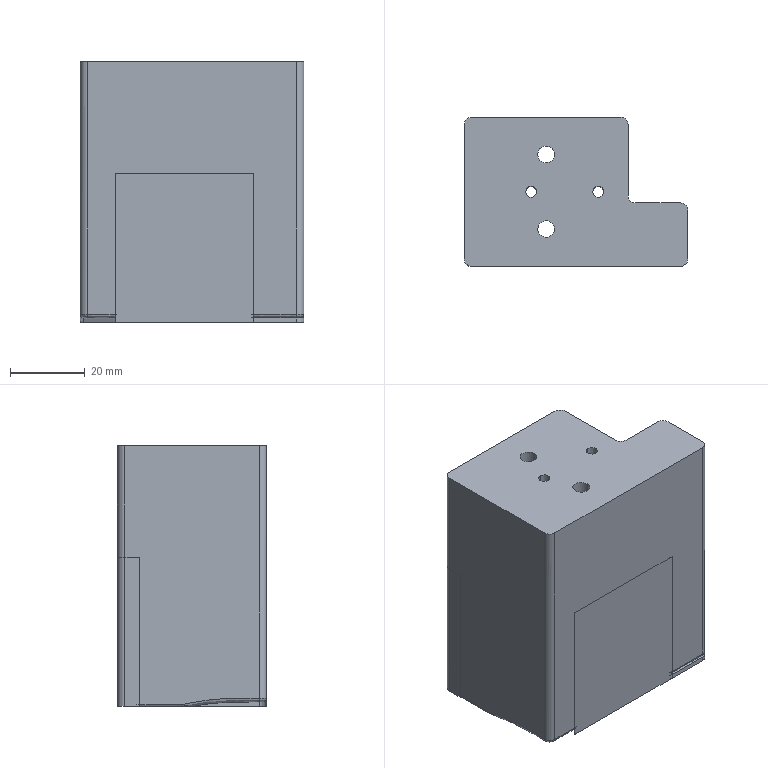NC program | NX | posted with a generic post | part box 60.004 x 40.015 x 70 mm
Lines 1319 to 2490 of 2490:
(ZLEVEL_PROFILE_COPY , TOOL : D6R0.5)
N2612 T08 M6
N2614 G54
N2616 G17 G0 G90 X-39.204 Y31.66 B0. C0. S9500 M3
N2618 G43 Z30. H8
N2620 Z1.491
N2622 G94 G1 Z-0.009 F1000.
N2624 X-38.808 Y30.909
N2626 G3 X-38.3 Y30.589 R0.6
N2628 X-35. Y30.711 R21.969 F3000.
N2630 G1 X35.
N2632 G3 X38.301 Y30.583 R28.78
N2634 G1 Y30.622 Z-0.014
N2636 Y30.645 Z-0.018
N2638 G2 X35. Y30.802 R29.046
N2640 G1 X-35.
N2642 G2 X-38.3 Y30.657 R19.705
N2644 G1 Y30.696 Z-0.024
N2646 Y30.722 Z-0.029
N2648 G3 X-35. Y30.878 R17.937
N2650 G1 X35.
N2652 G3 X38.3 Y30.71 R25.062
N2654 G1 Y30.75 Z-0.035
N2656 Y30.766 Z-0.042
N2658 G2 X35. Y30.954 R25.313
N2660 G1 X-35.
N2662 G2 X-38.3 Y30.78 R16.894
N2664 G1 Y30.838 Z-0.049
N2666 Y30.851 Z-0.057
N2668 G3 X-35. Y31.03 R17.218
N2670 G1 X35.
N2672 G3 X38.3 Y30.835 R25.117
N2674 G1 Y30.892 Z-0.066
N2676 Y30.914 Z-0.075
N2678 G2 X35. Y31.107 R26.565
N2680 G1 X-35.
N2682 G2 X-38.3 Y30.934 R19.629
N2684 G1 Y30.99 Z-0.085
N2686 Y31.028 Z-0.095
N2688 G3 X-35. Y31.184 R20.824
N2690 G1 X35.
N2692 X35.591 Y31.116
N2694 X38.3 Y31.005
N2696 Y31.052 Z-0.107
N2698 Y31.092 Z-0.119
N2700 G2 X35. Y31.262 R23.577
N2702 G1 X-35.
N2704 G2 X-38.3 Y31.107 R20.444
N2706 G1 Y31.15 Z-0.133
N2708 Y31.193 Z-0.146
N2710 G3 X-35. Y31.343 R22.3
N2712 G1 X35.
N2714 G3 X38.3 Y31.183 R24.663
N2716 G1 Y31.235 Z-0.162
N2718 Y31.286 Z-0.178
N2720 G2 X35. Y31.426 R29.09
N2722 G1 X-35.
N2724 G2 X-38.3 Y31.292 R27.305
N2726 G1 Y31.347 Z-0.195
N2728 Y31.395 Z-0.213
N2730 G3 X-35. Y31.51 R27.18
N2732 G1 X35.
N2734 G3 X38.3 Y31.395 R27.678
N2736 G1 Y31.445 Z-0.232
N2738 Y31.473 Z-0.252
N2740 G2 X35. Y31.594 R26.126
N2742 G1 X-35.
N2744 G2 X-38.3 Y31.474 R25.707
N2746 G1 Y31.532 Z-0.273
N2748 Y31.559 Z-0.294
N2750 G3 X-35. Y31.677 R26.757
N2752 G1 X35.
N2754 G3 X38.3 Y31.559 R26.83
N2756 G1 Y31.615 Z-0.317
N2758 Y31.652 Z-0.34
N2760 G2 X35. Y31.759 R30.651
N2762 G1 X-35.
N2764 G2 X-38.3 Y31.652 R30.623
N2766 G1 Y31.704 Z-0.365
N2768 Y31.748 Z-0.39
N2770 G3 X-35. Y31.841 R36.413
N2772 G1 X35.
N2774 G3 X38.3 Y31.748 R36.471
N2776 G1 Y31.799 Z-0.416
N2778 Y31.84 Z-0.443
N2780 G2 X35. Y31.921 R45.745
N2782 G1 X-35.
N2784 G2 X-38.3 Y31.84 R45.528
N2786 G1 Y31.884 Z-0.471
N2788 Y31.925 Z-0.5
N2790 G3 X-35. Y32. R42.31
N2792 G1 X35.
N2794 G3 X38.3 Y31.925 R42.219
N2796 G1 Y31.962 Z-0.53
N2798 Y31.998 Z-0.56
N2800 G2 X35. Y32.076 R40.059
N2802 G1 X-35.
N2804 G2 X-38.3 Y31.998 R40.061
N2806 G1 Y32.037 Z-0.591
N2808 Y32.075 Z-0.623
N2810 G3 X-35. Y32.151 R41.473
N2812 G1 X35.
N2814 G3 X38.3 Y32.075 R41.472
N2816 G1 Y32.116 Z-0.656
N2818 Y32.154 Z-0.689
N2820 G2 X35. Y32.223 R48.13
N2822 G1 X-35.
N2824 G2 X-38.3 Y32.154 R48.064
N2826 G1 Y32.195 Z-0.724
N2828 Y32.236 Z-0.758
N2830 G3 X-35. Y32.293 R55.16
N2832 G1 X35.
N2834 G3 X38.3 Y32.236 R55.158
N2836 G1 Y32.267 Z-0.794
N2838 Y32.297 Z-0.83
N2840 G2 X35. Y32.361 R48.287
N2842 G1 X-35.
N2844 G2 X-38.3 Y32.297 R48.288
N2846 G1 Y32.331 Z-0.868
N2848 Y32.36 Z-0.905
N2850 G3 X-35. Y32.425 R47.821
N2852 G1 X35.
N2854 G3 X38.3 Y32.36 R47.819
N2856 G1 Y32.393 Z-0.944
N2858 Y32.423 Z-0.983
N2860 G2 X35. Y32.487 R49.662
N2862 G1 X-35.
N2864 G2 X-38.3 Y32.423 R49.664
N2866 G1 Y32.458 Z-1.023
N2868 Y32.483 Z-1.063
N2870 G3 X-35. Y32.545 R52.544
N2872 G1 X35.
N2874 G3 X38.3 Y32.483 R52.542
N2876 G1 Y32.52 Z-1.104
N2878 Y32.545 Z-1.145
N2880 G2 X35. Y32.601 R66.305
N2882 G1 X-35.
N2884 G2 X-38.3 Y32.545 R66.306
N2886 G1 Y32.574 Z-1.187
N2888 Y32.599 Z-1.23
N2890 G3 X-35. Y32.653 R58.914
N2892 G1 X35.
N2894 G3 X38.3 Y32.599 R59.147
N2896 G1 Y32.623 Z-1.273
N2898 Y32.646 Z-1.316
N2900 G2 X35. Y32.702 R54.272
N2902 G1 X-35.
N2904 G2 X-38.3 Y32.646 R54.274
N2906 G1 Y32.67 Z-1.361
N2908 Y32.693 Z-1.405
N2910 G3 X-35. Y32.747 R57.595
N2912 G1 X35.
N2914 G3 X38.3 Y32.693 R57.593
N2916 G1 Y32.718 Z-1.45
N2918 Y32.741 Z-1.496
N2920 G2 X35. Y32.789 R68.133
N2922 G1 X-35.
N2924 G2 X-38.3 Y32.741 R68.262
N2926 G1 Y32.761 Z-1.542
N2928 Y32.774 Z-1.588
N2930 G3 X-35. Y32.828 R69.805
N2932 G1 X35.
N2934 X36.627 Y32.776
N2936 X38.3 Y32.775
N2938 Y32.796 Z-1.635
N2940 Y32.808 Z-1.681
N2942 G2 X35. Y32.862 R62.375
N2944 G1 X-35.
N2946 G2 X-38.3 Y32.805 R65.941
N2948 G1 Y32.827 Z-1.729
N2950 Y32.838 Z-1.776
N2952 G3 X-35. Y32.893 R71.079
N2954 G1 X35.
N2956 G3 X38.3 Y32.841 R61.18
N2958 G1 Y32.859 Z-1.824
N2960 Y32.874 Z-1.873
N2962 G2 X35. Y32.92 R65.916
N2964 G1 X-35.
N2966 G2 X-38.3 Y32.87 R75.705
N2968 G1 Y32.885 Z-1.921
N2970 Y32.896 Z-1.97
N2972 G3 X-35. Y32.943 R90.31
N2974 G1 X35.
N2976 G3 X38.3 Y32.901 R76.7
N2978 G1 Y32.918 Z-2.019
N2980 Y32.928 Z-2.068
N2982 G2 X35. Y32.962 R88.257
N2984 G1 X-35.
N2986 G2 X-38.301 Y32.923 R128.489
N2988 G1 Y32.935 Z-2.117
N2990 Y32.945 Z-2.167
N2992 G3 X-35. Y32.978 R137.834
N2994 G1 X35.
N2996 G3 X38.3 Y32.948 R92.566
N2998 G1 Y32.96 Z-2.208
N3000 Y32.962 Z-2.25
N3002 G2 X35.591 Y32.97 R356.718
N3004 G1 X35. Y32.987
N3006 X-35.
N3008 G2 X-38.301 Y32.96 R156.374
N3010 G1 Y32.968 Z-2.292
N3012 X-38.3 Y32.976 Z-2.333
N3014 X-35.245 Y32.988
N3016 X-35. Y32.994
N3018 X35.
N3020 X35.591 Y32.982
N3022 X38.3 Y32.977
N3024 Y32.985 Z-2.375
N3026 Y32.992 Z-2.417
N3028 X35.245 Y32.995
N3030 X35. Y32.999
N3032 X-35.
N3034 X-38.3 Y32.991
N3036 X-38.298 Y32.999 Z-2.5
N3038 X38.298
N3040 G3 X38.817 Y33.299 R0.6
N3042 G1 X39.272 Y34.085
N3044 Z-1.
N3046 G0 Z30.
N3048 X39.204 Y-15.66
N3050 Z1.491
N3052 G1 Z-0.009 F1000.
N3054 X38.808 Y-14.909
N3056 G3 X38.3 Y-14.589 R0.6
N3058 X35. Y-14.711 R21.968 F3000.
N3060 G1 X-35.
N3062 G3 X-38.301 Y-14.583 R28.779
N3064 G1 Y-14.622 Z-0.014
N3066 Y-14.645 Z-0.018
N3068 G2 X-35. Y-14.802 R29.046
N3070 G1 X35.
N3072 G2 X38.3 Y-14.657 R19.704
N3074 G1 Y-14.696 Z-0.024
N3076 Y-14.722 Z-0.029
N3078 G3 X35. Y-14.878 R17.936
N3080 G1 X-35.
N3082 G3 X-38.3 Y-14.71 R25.063
N3084 G1 Y-14.75 Z-0.035
N3086 Y-14.766 Z-0.042
N3088 G2 X-35. Y-14.954 R25.314
N3090 G1 X35.
N3092 G2 X38.3 Y-14.78 R16.894
N3094 G1 Y-14.838 Z-0.049
N3096 Y-14.851 Z-0.057
N3098 G3 X35. Y-15.03 R17.217
N3100 G1 X-35.
N3102 G3 X-38.3 Y-14.835 R25.117
N3104 G1 Y-14.892 Z-0.066
N3106 Y-14.914 Z-0.075
N3108 G2 X-35. Y-15.107 R26.566
N3110 G1 X35.
N3112 G2 X38.3 Y-14.934 R19.629
N3114 G1 Y-14.99 Z-0.085
N3116 Y-15.028 Z-0.095
N3118 G3 X35. Y-15.184 R20.824
N3120 G1 X-35.
N3122 X-35.591 Y-15.116
N3124 X-38.3 Y-15.005
N3126 Y-15.052 Z-0.107
N3128 Y-15.092 Z-0.119
N3130 G2 X-35. Y-15.262 R23.578
N3132 G1 X35.
N3134 G2 X38.3 Y-15.107 R20.443
N3136 G1 Y-15.15 Z-0.133
N3138 Y-15.193 Z-0.146
N3140 G3 X35. Y-15.343 R22.3
N3142 G1 X-35.
N3144 G3 X-38.3 Y-15.183 R24.664
N3146 G1 Y-15.235 Z-0.162
N3148 Y-15.286 Z-0.178
N3150 G2 X-35. Y-15.426 R29.091
N3152 G1 X35.
N3154 G2 X38.3 Y-15.292 R27.305
N3156 G1 Y-15.347 Z-0.195
N3158 Y-15.395 Z-0.213
N3160 G3 X35. Y-15.51 R27.179
N3162 G1 X-35.
N3164 G3 X-38.3 Y-15.395 R27.679
N3166 G1 Y-15.445 Z-0.232
N3168 Y-15.473 Z-0.252
N3170 G2 X-35. Y-15.594 R26.127
N3172 G1 X35.
N3174 G2 X38.3 Y-15.474 R25.706
N3176 G1 Y-15.532 Z-0.273
N3178 Y-15.559 Z-0.294
N3180 G3 X35. Y-15.677 R26.756
N3182 G1 X-35.
N3184 G3 X-38.3 Y-15.559 R26.831
N3186 G1 Y-15.615 Z-0.317
N3188 Y-15.652 Z-0.34
N3190 G2 X-35. Y-15.759 R30.652
N3192 G1 X35.
N3194 G2 X38.3 Y-15.652 R30.622
N3196 G1 Y-15.704 Z-0.365
N3198 Y-15.748 Z-0.39
N3200 G3 X35. Y-15.841 R36.412
N3202 G1 X-35.
N3204 G3 X-38.3 Y-15.748 R36.472
N3206 G1 Y-15.799 Z-0.416
N3208 Y-15.84 Z-0.443
N3210 G2 X-35. Y-15.921 R45.746
N3212 G1 X35.
N3214 G2 X38.3 Y-15.84 R45.526
N3216 G1 Y-15.884 Z-0.471
N3218 Y-15.925 Z-0.5
N3220 G3 X35. Y-16. R42.309
N3222 G1 X-35.
N3224 G3 X-38.3 Y-15.925 R42.22
N3226 G1 Y-15.962 Z-0.53
N3228 Y-15.998 Z-0.56
N3230 G2 X-35. Y-16.076 R40.061
N3232 G1 X35.
N3234 G2 X38.3 Y-15.998 R40.059
N3236 G1 Y-16.037 Z-0.591
N3238 Y-16.075 Z-0.623
N3240 G3 X35. Y-16.151 R41.472
N3242 G1 X-35.
N3244 G3 X-38.3 Y-16.075 R41.473
N3246 G1 Y-16.116 Z-0.656
N3248 Y-16.154 Z-0.689
N3250 G2 X-35. Y-16.223 R48.132
N3252 G1 X35.
N3254 G2 X38.3 Y-16.154 R48.062
N3256 G1 Y-16.195 Z-0.724
N3258 Y-16.236 Z-0.758
N3260 G3 X35. Y-16.293 R55.158
N3262 G1 X-35.
N3264 G3 X-38.3 Y-16.236 R55.16
N3266 G1 Y-16.267 Z-0.794
N3268 Y-16.297 Z-0.83
N3270 G2 X-35. Y-16.361 R48.288
N3272 G1 X35.
N3274 G2 X38.3 Y-16.297 R48.287
N3276 G1 Y-16.331 Z-0.868
N3278 Y-16.36 Z-0.905
N3280 G3 X35. Y-16.425 R47.819
N3282 G1 X-35.
N3284 G3 X-38.3 Y-16.36 R47.821
N3286 G1 Y-16.393 Z-0.944
N3288 Y-16.423 Z-0.983
N3290 G2 X-35. Y-16.487 R49.664
N3292 G1 X35.
N3294 G2 X38.3 Y-16.423 R49.662
N3296 G1 Y-16.458 Z-1.023
N3298 Y-16.483 Z-1.063
N3300 G3 X35. Y-16.545 R52.542
N3302 G1 X-35.
N3304 G3 X-38.3 Y-16.483 R52.544
N3306 G1 Y-16.52 Z-1.104
N3308 Y-16.545 Z-1.145
N3310 G2 X-35. Y-16.601 R66.306
N3312 G1 X35.
N3314 G2 X38.3 Y-16.545 R66.305
N3316 G1 Y-16.574 Z-1.187
N3318 Y-16.599 Z-1.23
N3320 G3 X35. Y-16.653 R58.912
N3322 G1 X-35.
N3324 G3 X-38.3 Y-16.599 R59.149
N3326 G1 Y-16.623 Z-1.273
N3328 Y-16.646 Z-1.316
N3330 G2 X-35. Y-16.702 R54.274
N3332 G1 X35.
N3334 G2 X38.3 Y-16.646 R54.272
N3336 G1 Y-16.67 Z-1.361
N3338 Y-16.693 Z-1.405
N3340 G3 X35. Y-16.747 R57.593
N3342 G1 X-35.
N3344 G3 X-38.3 Y-16.693 R57.595
N3346 G1 Y-16.718 Z-1.45
N3348 Y-16.741 Z-1.496
N3350 G2 X-35. Y-16.789 R70.332
N3352 G1 X35.
N3354 G2 X38.3 Y-16.741 R68.944
N3356 G1 Y-16.764 Z-1.542
N3358 X38.301 Y-16.775 Z-1.588
N3360 G2 X36.973 Y-16.776 R23.942
N3362 G1 X36.627 Y-16.778
N3364 X35. Y-16.828
N3366 X-35.
N3368 G3 X-38.3 Y-16.775 R72.311
N3370 G1 Y-16.799 Z-1.635
N3372 X-38.301 Y-16.808 Z-1.681
N3374 G2 X-35. Y-16.862 R68.249
N3376 G1 X35.
N3378 X35.245 Y-16.852
N3380 X36.627 Y-16.813
N3382 X36.973 Y-16.81
N3384 G3 X38.301 Y-16.806 R39.492
N3386 G1 Y-16.827 Z-1.729
N3388 Y-16.838 Z-1.776
N3390 G3 X35. Y-16.893 R74.971
N3392 G1 X-35.
N3394 G3 X-38.301 Y-16.841 R65.626
N3396 G1 X-38.3 Y-16.859 Z-1.824
N3398 Y-16.874 Z-1.873
N3400 G2 X-35. Y-16.92 R66.405
N3402 G1 X35.
N3404 G2 X38.3 Y-16.87 R76.655
N3406 G1 Y-16.885 Z-1.921
N3408 X38.301 Y-16.897 Z-1.97
N3410 G3 X35. Y-16.943 R111.278
N3412 G1 X-35.
N3414 G3 X-38.301 Y-16.901 R88.915
N3416 G1 Y-16.915 Z-2.019
N3418 Y-16.928 Z-2.068
N3420 G2 X-35. Y-16.962 R93.145
N3422 G1 X35.
N3424 G2 X38.301 Y-16.923 R141.736
N3426 G1 X38.302 Y-16.935 Z-2.117
N3428 Y-16.945 Z-2.167
N3430 X35.591 Y-16.966
N3432 X35. Y-16.978
N3434 X-35.
N3436 G3 X-38.303 Y-16.948 R139.014
N3438 G1 Y-16.956 Z-2.208
N3440 Y-16.963 Z-2.25
N3442 G2 X-35. Y-16.987 R166.106
N3444 G1 X35.
N3446 X35.245 Y-16.979
N3448 X38.303 Y-16.961
N3450 X38.302 Y-16.968 Z-2.292
N3452 Y-16.976 Z-2.333
N3454 X35.245 Y-16.988
N3456 X35. Y-16.994
N3458 X-35.
N3460 X-35.245 Y-16.989
N3462 X-38.302 Y-16.977
N3464 X-38.301 Y-16.984 Z-2.375
N3466 Y-16.992 Z-2.417
N3468 X-35.245 Y-16.995
N3470 X-35. Y-16.999
N3472 X35.
N3474 X38.301 Y-16.991
N3476 X38.299 Y-16.998 Z-2.5
N3478 X-38.299
N3480 G3 X-38.819 Y-17.298 R0.6
N3482 G1 X-39.273 Y-18.084
N3484 Z-1.
N3486 G0 Z30.
(ZLEVEL_PROFILE_COPY_COPY_1 , TOOL : D6R0.5)
N3488 X39.23 Y-18.097
N3490 Z-19.6
N3492 G1 Z-21.1 F1000.
N3494 X38.77 Y-17.3
N3496 G3 X38.25 Y-17. R0.6
N3498 G1 X-38.252 F3000.
N3500 X-38.26 Z-21.2
N3502 X38.258
N3504 X38.267 Z-21.3
N3506 X-38.268
N3508 X-38.277 Z-21.4
N3510 X38.275
N3512 X38.283 Y-17.006 Z-21.5
N3514 X35.245 Y-17.003
N3516 X34.9 Y-17.
N3518 X-34.9
N3520 X-38.285 Y-17.008
N3522 X-38.293 Y-17.027 Z-21.6
N3524 G3 X-34.554 Y-17.003 R313.635
N3526 G1 X-5.097
N3528 X-5.01 Y-17.009
N3530 X-5. Y-17.003
N3532 X34.9
N3534 G3 X38.292 Y-17.024 R118.309
N3536 G1 X38.3 Y-17.043 Z-21.699
N3538 G2 X35. Y-17.013 R80.934
N3540 G1 X-35.
N3542 G2 X-38.3 Y-17.048 R133.603
N3544 G1 Y-17.063 Z-21.748
N3546 Y-17.077 Z-21.797
N3548 G3 X-34.9 Y-17.03 R96.823
N3550 G1 X-5.097
N3552 X-5.01 Y-17.035
N3554 X-5. Y-17.03
N3556 X34.9
N3558 G3 X38.3 Y-17.072 R71.415
N3560 G1 Y-17.085 Z-21.846
N3562 Y-17.102 Z-21.894
N3564 G2 X35.245 Y-17.07 R69.623
N3566 G1 X34.836 Y-17.058
N3568 X34.822 Y-17.053
N3570 X-4.811
N3572 X-4.838 Y-17.058
N3574 X-5.14 Y-17.06
N3576 X-5.189 Y-17.053
N3578 X-34.812
N3580 X-34.878 Y-17.061
N3582 X-36.292 Y-17.091
N3584 G2 X-38.3 Y-17.105 R68.304
N3586 G1 Y-17.118 Z-21.942
N3588 Y-17.133 Z-21.989
N3590 G3 X-36.282 Y-17.123 R63.448
N3592 G1 X-35.591 Y-17.106
N3594 X-35.245 Y-17.099
N3596 X-34.878 Y-17.092
N3598 X-34.812 Y-17.082
N3600 X-5.19
N3602 X-5.14 Y-17.091
N3604 X-4.821 Y-17.086
N3606 X-4.81 Y-17.082
N3608 X34.819
N3610 X34.862 Y-17.092
N3612 X36.487 Y-17.125
N3614 G3 X38.3 Y-17.132 R53.385
N3616 G1 Y-17.146 Z-22.036
N3618 Y-17.173 Z-22.082
N3620 G2 X34.86 Y-17.118 R62.25
N3622 G1 X-34.856
N3624 X-36.627 Y-17.174
N3626 X-38.3 Y-17.167
N3628 Y-17.191 Z-22.127
N3630 Y-17.214 Z-22.172
N3632 G3 X-34.812 Y-17.159 R61.071
N3634 G1 X-5.191
N3636 X-5.14 Y-17.166
N3638 X-4.838 Y-17.165
N3640 X-4.809 Y-17.159
N3642 X34.812
N3644 G3 X38.3 Y-17.214 R60.08
N3646 G1 Y-17.238 Z-22.216
N3648 Y-17.263 Z-22.259
N3650 G2 X34.808 Y-17.206 R58.888
N3652 G1 X-4.808
N3654 X-4.838 Y-17.211
N3656 X-5.14 Y-17.212
N3658 X-5.192 Y-17.206
N3660 X-34.812
N3662 G2 X-38.3 Y-17.263 R58.665
N3664 G1 Y-17.283 Z-22.301
N3666 Y-17.314 Z-22.342
N3668 G3 X-34.796 Y-17.259 R62.267
N3670 G1 X-5.193
N3672 X-5.14 Y-17.267
N3674 X-4.807 Y-17.259
N3676 X34.804
N3678 G3 X38.3 Y-17.314 R61.659
N3680 G1 Y-17.347 Z-22.382
N3682 Y-17.379 Z-22.421
N3684 G2 X34.799 Y-17.316 R53.507
N3686 G1 X-4.795
N3688 X-4.838 Y-17.324
N3690 X-5.14 Y-17.325
N3692 X-5.205 Y-17.316
N3694 X-34.796
N3696 G2 X-38.3 Y-17.379 R53.656
N3698 G1 Y-17.41 Z-22.459
N3700 Y-17.452 Z-22.496
N3702 G3 X-34.812 Y-17.378 R46.03
N3704 G1 X34.808
N3706 G3 X38.3 Y-17.452 R42.403
N3708 G1 Y-17.479 Z-22.531
N3710 Y-17.52 Z-22.566
N3712 G2 X34.9 Y-17.462 R56.275
N3714 G1 X34.837 Y-17.445
N3716 X-4.801
N3718 X-4.838 Y-17.459
N3720 X-5.2 Y-17.445
N3722 X-34.839
N3724 X-34.9 Y-17.462
N3726 G2 X-38.3 Y-17.52 R56.277
N3728 G1 Y-17.552 Z-22.598
N3730 Y-17.594 Z-22.631
N3732 G3 X-34.778 Y-17.514 R44.648
N3734 G1 X-5.221
N3736 X-5.188 Y-17.526
N3738 X-4.814
N3740 X-4.783 Y-17.514
N3742 X34.782
N3744 G3 X38.3 Y-17.594 R44.469
N3746 G1 Y-17.628 Z-22.661
N3748 Y-17.672 Z-22.69
N3750 G2 X34.786 Y-17.587 R39.562
N3752 G1 X-4.785
N3754 X-4.816 Y-17.601
N3756 X-5.183
N3758 X-5.209 Y-17.587
N3760 X-34.785
N3762 G2 X-38.3 Y-17.672 R39.602
N3764 G1 Y-17.71 Z-22.717
N3766 Y-17.75 Z-22.744
N3768 G3 X-34.847 Y-17.662 R33.374
N3770 G1 X-5.197
N3772 X-4.838 Y-17.678
N3774 X-4.808 Y-17.662
N3776 X34.848
N3778 G3 X38.3 Y-17.75 R32.893
N3780 G1 Y-17.796 Z-22.768
N3782 Y-17.84 Z-22.792
N3784 G2 X34.727 Y-17.739 R35.264
N3786 G1 X-34.775
N3788 G2 X-38.3 Y-17.84 R33.761
N3790 G1 Y-17.88 Z-22.813
N3792 Y-17.929 Z-22.834
N3794 G3 X-34.748 Y-17.815 R35.258
N3796 G1 X-5.218
N3798 X-5.183 Y-17.829
N3800 X-4.838 Y-17.83
N3802 X-4.786 Y-17.815
N3804 X34.727
N3806 G3 X38.3 Y-17.93 R36.846
N3808 G1 Y-17.972 Z-22.852
N3810 Y-18.026 Z-22.87
N3812 G2 X34.727 Y-17.889 R31.359
N3814 G1 X-34.892
N3816 G2 X-38.3 Y-18.021 R23.99
N3818 G1 Y-18.058 Z-22.884
N3820 Y-18.109 Z-22.899
N3822 G3 X-34.845 Y-17.959 R22.16
N3824 G1 X-5.14
N3826 X-5.01 Y-17.988
N3828 X-4.848 Y-17.959
N3830 X34.724
N3832 G3 X38.203 Y-18.119 R28.399
N3834 G1 X38.202 Y-18.154 Z-22.911
N3836 Y-18.206 Z-22.923
N3838 G2 X34.718 Y-18.026 R25.496
N3840 G1 X-4.72
N3842 X-4.769 Y-18.047
N3844 X-5.234 Y-18.046
N3846 X-5.29 Y-18.026
N3848 X-34.718
N3850 G2 X-38.299 Y-18.196 R23.231
N3852 G1 Y-18.213 Z-22.933
N3854 X-38.298 Y-18.265 Z-22.942
N3856 G3 X-34.681 Y-18.088 R24.528
N3858 G1 X34.679
N3860 G3 X38.201 Y-18.275 R25.639
N3862 G1 Y-18.289 Z-22.949
N3864 X38.2 Y-18.327 Z-22.956
N3866 G2 X34.63 Y-18.141 R28.935
N3868 G1 X-34.631
N3870 G2 X-38.298 Y-18.317 R25.974
N3872 G1 Y-18.323 Z-22.962
N3874 Y-18.358 Z-22.968
N3876 G3 X-35. Y-18.192 R17.285
N3878 G1 X35.
N3880 X35.562 Y-18.272
N3882 X35.591 Y-18.29
N3884 G3 X38.2 Y-18.369 R42.051
N3886 G1 X38.269 Y-18.414 Z-22.978
N3888 G2 X35. Y-18.245 R22.166
N3890 G1 X-35.
N3892 X-35.04 Y-18.283
N3894 X-35.091 Y-18.303
N3896 X-35.146
N3898 X-35.936 Y-18.37
N3900 X-38.297 Y-18.396
N3902 X-38.2 Y-18.483 Z-22.989
N3904 X-35.936 Y-18.476
N3906 X-35.591 Y-18.457
N3908 X-35. Y-18.322
N3910 X35.
N3912 G3 X38.267 Y-18.497 R21.667
N3914 G1 Y-18.511 Z-22.995
N3916 X38.265 Y-18.556 Z-23.
N3918 G2 X34.554 Y-18.422 R41.331
N3920 G1 X-34.209 Y-18.42
N3922 X-34.9 Y-18.501
N3924 X-38.01 Y-18.553
N3926 X-38.2
N3928 G3 X-38.72 Y-18.853 R0.6
N3930 G1 X-39.176 Y-19.643
N3932 Z-21.5
N3934 G0 Z30.
(ZLEVEL_PROFILE_COPY_COPY_1_COPY , TOOL : D6R0.5)
N3936 X37.451 Y-31.576
N3938 Z-21.505
N3940 G1 Z-23.005 F1000.
N3942 X36.933 Y-30.735
N3944 G3 X36.406 Y-30.45 R0.6
N3946 G1 X33.522 Y-30.531 F3000.
N3948 X33.105 Y-30.658
N3950 X-35.
N3952 G3 X-35.936 Y-30.498 R5.184
N3954 G1 X-36.282 Y-30.576
N3956 X-36.627 Y-30.554
N3958 X-38.3 Y-30.557
N3960 Y-30.601 Z-23.01
N3962 G3 X-35.59 Y-30.602 R62.171
N3964 G1 X-35. Y-30.723
N3966 X33.105
N3968 X33.522 Y-30.636
N3970 X36.405 Y-30.531
N3972 Y-30.645 Z-23.017
N3974 X33.105 Y-30.791
N3976 X-35.
N3978 G3 X-38.3 Y-30.636 R24.421
N3980 G1 Y-30.677 Z-23.025
N3982 G2 X-35. Y-30.853 R29.171
N3984 G1 X33.104
N3986 X33.176 Y-30.827
N3988 X36.404 Y-30.772
N3990 Y-30.811 Z-23.03
N3992 Y-30.826 Z-23.035
N3994 X33.176 Y-30.881
N3996 X33.104 Y-30.915
N3998 X-35.
N4000 G3 X-38.3 Y-30.726 R27.45
N4002 G1 Y-30.783 Z-23.046
N4004 G2 X-35. Y-30.98 R23.168
N4006 G1 X33.104
N4008 X33.176 Y-30.946
N4010 X36.403 Y-30.892
N4012 Y-30.963 Z-23.054
N4014 Y-30.974 Z-23.061
N4016 X33.176 Y-31.028
N4018 X33.103 Y-31.05
N4020 X-35.
N4022 G3 X-38.3 Y-30.847 R21.936
N4024 G1 Y-30.892 Z-23.07
N4026 Y-30.925 Z-23.079
N4028 G2 X-35. Y-31.124 R22.938
N4030 G1 X33.102
N4032 X36.402 Y-31.075
N4034 Y-31.11 Z-23.085
N4036 Y-31.129 Z-23.09
N4038 X33.176 Y-31.154
N4040 X33.102 Y-31.166
N4042 X-35.
N4044 G3 X-38.3 Y-30.973 R23.578
N4046 G1 Y-30.994 Z-23.095
N4048 G2 X-36.258 Y-31.063 R16.584
N4050 G1 X-35. Y-31.184
N4052 X33.102
N4054 X33.176 Y-31.169
N4056 X36.402 Y-31.148
N4058 Y-31.166 Z-23.098
N4060 Y-31.167 Z-23.1
N4062 X33.102 Y-31.201
N4064 X-35.
N4066 X-36.973 Y-31.026
N4068 X-38.3 Y-31.016
N4070 Y-31.038 Z-23.105
N4072 X-36.973 Y-31.046
N4074 X-35. Y-31.218
N4076 X33.101
N4078 X33.522 Y-31.207
N4080 X36.402 Y-31.186
N4082 Y-31.203 Z-23.108
N4084 Y-31.205 Z-23.11
N4086 X33.522 Y-31.224
N4088 X33.101 Y-31.234
N4090 X-35.
N4092 X-35.245 Y-31.205
N4094 X-36.973 Y-31.067
N4096 X-38.3 Y-31.059
N4098 Y-31.081 Z-23.115
N4100 X-36.973 Y-31.087
N4102 X-35.245 Y-31.22
N4104 X-35. Y-31.25
N4106 X33.101
N4108 X33.522 Y-31.242
N4110 X36.401 Y-31.224
N4112 G2 X36.923 Y-31.52 R0.6
N4114 G1 X37.378 Y-32.297
N4116 Z-21.615
N4118 G0 Z30.
N4120 X40.416 Y-24.462
N4122 Z-21.6
N4124 G1 Z-23.1 F1000.
N4126 X39.533 Y-24.958
N4128 G3 X39.227 Y-25.474 R0.6
N4130 G1 X39.209 Y-26.987 F3000.
N4132 G3 X39.503 Y-27.51 R0.6
N4134 G1 X40.402 Y-28.043
N4136 Z-21.6
N4138 G0 Z30.
N4140 X39.207 Y-28.037
N4142 Z-21.6
N4144 G1 Z-23.105 F1000.
N4146 G3 X39.44 Y-24.646 R8.662 F3000.
N4148 G2 X39.671 Y-24.092 R0.6
N4150 G1 X40.429 Y-23.513
N4152 Z-21.605
N4154 G0 Z30.
N4156 X40.805 Y-23.539
N4158 Z-21.61
N4160 G1 Z-23.11 F1000.
N4162 X40.154 Y-24.083
N4164 G3 X39.948 Y-24.646 R0.6
N4166 G2 X39.319 Y-28.712 R6.433 F3000.
N4168 G1 X39.026 Y-29.176
N4170 X38.997 Y-29.215
N4172 X38.999 Y-29.263
N4174 G3 X39.277 Y-29.795 R0.6
N4176 G1 X39.906 Y-30.194
N4178 Z-21.61
N4180 G0 Z30.
N4182 X38.884 Y-29.577
N4184 Z-21.61
N4186 G1 Z-23.115 F1000.
N4188 X39.883 Y-28.407 F3000.
N4190 G2 X40.449 Y-28.206 R0.6
N4192 G1 X41.229 Y-28.351
N4194 Z-21.615
N4196 G0 Z30.
N4198 X41.107 Y-29.228
N4200 Z-21.62
N4202 G1 Z-23.12 F1000.
N4204 X40.358 Y-28.995
N4206 G3 X39.773 Y-29.126 R0.6
N4208 G1 X39.742 Y-29.155 F3000.
N4210 X38.77 Y-29.826
N4212 X38.737 Y-29.881
N4214 G2 X36.401 Y-31.242 R2.727
N4216 G1 X33.522 Y-31.259
N4218 X33.101 Y-31.266
N4220 X-35.
N4222 G3 X-35.59 Y-31.216 R4.156
N4224 X-38.3 Y-31.103 R19.851
N4226 G1 Y-31.123 Z-23.126
N4228 G2 X-35.59 Y-31.234 R19.728
N4230 X-35. Y-31.282 R3.682
N4232 G1 X33.101
N4234 X33.522 Y-31.278
N4236 X36.401 Y-31.263
N4238 G3 X38.517 Y-30.219 R2.684
N4240 G1 X38.607 Y-30.107
N4242 X39.571 Y-29.519
N4244 G2 X40.171 Y-29.505 R0.6
N4246 G1 X40.898 Y-29.901
N4248 Z-21.626
N4250 G0 Z30.
N4252 X40.599 Y-30.473
N4254 Z-21.631
N4256 G1 Z-23.131 F1000.
N4258 X39.838 Y-29.973
N4260 G3 X39.239 Y-29.939 R0.6
N4262 G1 X38.438 Y-30.342 F3000.
N4264 G2 X36.401 Y-31.283 R2.697
N4266 G1 X33.522 Y-31.295
N4268 X33.101 Y-31.3
N4270 X-35.
N4272 G3 X-36.973 Y-31.148 R70.051
N4274 G1 X-38.3 Y-31.144
N4276 Y-31.167 Z-23.135
N4278 Y-31.171 Z-23.139
N4280 G2 X-35. Y-31.322 R30.396
N4282 G1 X33.1
N4284 X33.522 Y-31.314
N4286 X36.401 Y-31.303
N4288 G3 X38.098 Y-30.698 R2.697
N4290 G1 X38.893 Y-30.369
N4292 X38.823 Y-30.506 Z-23.143
N4294 X38.739 Y-30.61 Z-23.147
N4296 X38.649 Y-30.68 Z-23.15
N4298 X38.014 Y-30.803
N4300 X37.967 Y-30.828
N4302 G2 X36.4 Y-31.332 R2.638
N4304 G1 X33.1 Y-31.354
N4306 X-35.
N4308 G3 X-38.3 Y-31.212 R28.449
N4310 G1 Y-31.251 Z-23.158
N4312 Y-31.268 Z-23.166
N4314 G2 X-35. Y-31.395 R28.242
N4316 G1 X33.099
N4318 X36.4 Y-31.371
N4320 G3 X37.9 Y-30.922 R2.709
N4322 G1 X37.929 Y-30.897
N4324 X38.503 Y-30.87
N4326 X38.47 Y-30.97 Z-23.185
N4328 X38.36 Y-30.965
N4330 X37.819 Y-31.017
N4332 X37.779 Y-31.047
N4334 G2 X36.399 Y-31.421 R2.796
N4336 G1 X33.522 Y-31.437
N4338 X33.099 Y-31.444
N4340 X-35.
N4342 G3 X-38.3 Y-31.318 R25.799
N4344 G1 Y-31.374 Z-23.208
N4346 G2 X-35. Y-31.499 R25.783
N4348 G1 X33.098
N4350 X36.398 Y-31.475
N4352 G3 X37.666 Y-31.166 R2.806
N4354 G1 X38.43 Y-31.103
N4356 X38.421 Y-31.161 Z-23.222
N4358 X38.417 Y-31.189 Z-23.236
N4360 X37.621 Y-31.248
N4362 X37.611 Y-31.255
N4364 G2 X36.397 Y-31.532 R2.616
N4366 G1 X33.097 Y-31.56
N4368 X-35.
N4370 G3 X-38.3 Y-31.439 R26.849
N4372 G1 Y-31.476 Z-23.252
N4374 Y-31.513 Z-23.267
N4376 G2 X-35. Y-31.625 R30.151
N4378 G1 X33.096
N4380 X35.941 Y-31.609
N4382 X36.396 Y-31.597
N4384 G3 X37.539 Y-31.354 R2.372
N4386 G1 X37.569 Y-31.34
N4388 X38.403 Y-31.284
N4390 X38.393 Y-31.354 Z-23.285
N4392 X38.388 Y-31.392 Z-23.303
N4394 X37.51 Y-31.445
N4396 X37.502 Y-31.449
N4398 G2 X36.395 Y-31.666 R2.573
N4400 G1 X35.941 Y-31.676
N4402 X33.176 Y-31.688
N4404 X33.095 Y-31.692
N4406 X-35.
N4408 G3 X-38.3 Y-31.596 R37.005
N4410 G1 Y-31.637 Z-23.322
N4412 Y-31.669 Z-23.342
N4414 G2 X-35. Y-31.762 R35.555
N4416 G1 X33.094
N4418 X33.176 Y-31.758
N4420 X36.394 Y-31.742
N4422 G3 X37.435 Y-31.545 R2.895
N4424 G1 X37.473 Y-31.53
N4426 X38.377 Y-31.493
N4428 X38.373 Y-31.545 Z-23.363
N4430 X38.37 Y-31.583 Z-23.385
N4432 X37.434 Y-31.62
N4434 X37.428 Y-31.623
N4436 G2 X36.393 Y-31.818 R2.747
N4438 G1 X33.093 Y-31.832
N4440 X-35.
N4442 G3 X-38.3 Y-31.74 R36.337
N4444 G1 Y-31.781 Z-23.408
N4446 Y-31.815 Z-23.431
N4448 G2 X-35. Y-31.903 R35.848
N4450 G1 X33.091
N4452 X33.176 Y-31.899
N4454 X36.391 Y-31.884
N4456 G3 X37.357 Y-31.722 R2.773
N4458 G1 X37.494 Y-31.702
N4460 X38.363 Y-31.68
N4462 X38.359 Y-31.731 Z-23.456
N4464 X38.356 Y-31.776 Z-23.481
N4466 X37.323 Y-31.801
N4468 X37.29 Y-31.812
N4470 G2 X36.39 Y-31.957 R3.142
N4472 G1 X33.09 Y-31.975
N4474 X-35.
N4476 G3 X-38.3 Y-31.89 R37.827
N4478 G1 Y-31.93 Z-23.508
N4480 Y-31.97 Z-23.535
N4482 G2 X-35. Y-32.046 R43.722
N4484 G1 X33.089
N4486 X33.176 Y-32.041
N4488 X36.388 Y-32.025
N4490 G3 X37.246 Y-31.897 R2.653
N4492 G1 X37.323 Y-31.881
N4494 X38.352 Y-31.86
N4496 X38.35 Y-31.905 Z-23.564
N4498 X38.349 Y-31.946 Z-23.593
N4500 X37.284 Y-31.962
N4502 X37.211 Y-31.978
N4504 G2 X36.387 Y-32.097 R2.808
N4506 G1 X33.176 Y-32.113
N4508 X33.087 Y-32.116
N4510 X-35.
N4512 G3 X-38.3 Y-32.053 R52.223
N4514 G1 Y-32.084 Z-23.623
N4516 Y-32.118 Z-23.653
N4518 G2 X-35. Y-32.185 R49.363
N4520 G1 X33.085
N4522 X33.115 Y-32.184
N4524 X33.176 Y-32.181
N4526 X36.385 Y-32.167
N4528 G3 X37.165 Y-32.06 R2.824
N4530 G1 X37.293 Y-32.04
N4532 X38.345 Y-32.026
N4534 X38.342 Y-32.071 Z-23.685
N4536 X38.34 Y-32.106 Z-23.717
N4538 X37.178 Y-32.127
N4540 X37.126 Y-32.141
N4542 G2 X36.383 Y-32.234 R3.334
N4544 G1 X33.153 Y-32.249
N4546 X33.083 Y-32.253
N4548 X-35.
N4550 G3 X-38.3 Y-32.183 R44.884
N4552 G1 Y-32.217 Z-23.751
N4554 Y-32.25 Z-23.784
N4556 G2 X-35. Y-32.318 R46.37
N4558 G1 X33.1
N4560 X33.176 Y-32.317
N4562 X36.382 Y-32.304
N4564 G3 X37.087 Y-32.219 R3.925
N4566 G1 X37.185 Y-32.197
N4568 X38.337 Y-32.182
N4570 X38.336 Y-32.223 Z-23.819
N4572 X38.335 Y-32.256 Z-23.854
N4574 X37.185 Y-32.271
N4576 X37.116 Y-32.27
N4578 X37.072 Y-32.287
N4580 X37.064
N4582 G2 X36.38 Y-32.367 R2.548
N4584 G1 X33.149 Y-32.379
N4586 X33.079 Y-32.382
N4588 X-35.
N4590 G3 X-38.3 Y-32.32 R52.348
N4592 G1 Y-32.355 Z-23.891
N4594 Y-32.39 Z-23.927
N4596 G2 X-35. Y-32.443 R63.469
N4598 G1 X33.077
N4600 X36.377 Y-32.432
N4602 G3 X37.043 Y-32.36 R2.985
N4604 G1 X37.078 Y-32.337
N4606 X37.119 Y-32.342
N4608 X38.332 Y-32.329
N4610 X38.331 Y-32.364 Z-23.965
N4612 X38.33 Y-32.394 Z-24.003
N4614 X37.185 Y-32.406
N4616 X37.116 Y-32.403
N4618 X37.04 Y-32.42
N4620 G2 X36.375 Y-32.496 R3.205
N4622 G1 X33.176 Y-32.499
N4624 X33.075 Y-32.502
N4626 X-35.
N4628 G3 X-38.3 Y-32.445 R57.029
N4630 G1 Y-32.473 Z-24.042
N4632 Y-32.499 Z-24.081
N4634 G2 X-35. Y-32.558 R52.175
N4636 G1 X33.073
N4638 X33.176 Y-32.552
N4640 X36.373 Y-32.547
N4642 G3 X36.963 Y-32.494 R3.213
N4644 G1 X37.006 Y-32.486
N4646 X37.064 Y-32.475
N4648 X38.327 Y-32.461
N4650 X38.326 Y-32.493 Z-24.122
N4652 X38.325 Y-32.52 Z-24.162
N4654 X37.047 Y-32.531
N4656 X36.889 Y-32.559
N4658 X36.451 Y-32.6
N4660 X36.371
N4662 X33.176 Y-32.606
N4664 X33.071 Y-32.612
N4666 X-35.
N4668 G3 X-38.3 Y-32.553 R53.246
N4670 G1 Y-32.582 Z-24.203
N4672 Y-32.609 Z-24.245
N4674 G2 X-35. Y-32.662 R62.731
N4676 G1 X33.068
N4678 X33.176 Y-32.66
N4680 X36.369 Y-32.654
N4682 G3 X36.858 Y-32.613 R3.281
N4684 G1 X37.021 Y-32.587
N4686 X38.323 Y-32.575
N4688 X38.322 Y-32.607 Z-24.288
N4690 X38.321 Y-32.632 Z-24.33
N4692 X37.047 Y-32.643
N4694 X37.032 Y-32.639
N4696 X36.828 Y-32.668
N4698 X36.455 Y-32.703
N4700 X36.367
N4702 X33.176 Y-32.707
N4704 X33.066 Y-32.71
N4706 X-35.
N4708 G3 X-38.3 Y-32.661 R62.031
N4710 G1 Y-32.681 Z-24.374
N4712 Y-32.7 Z-24.418
N4714 G2 X-35. Y-32.754 R54.903
N4716 G1 X33.064
N4718 X33.176 Y-32.751
N4720 X36.365 Y-32.75
N4722 G3 X36.896 Y-32.703 R2.738
N4724 G1 X37.043 Y-32.692
N4726 X37.116 Y-32.691
N4728 X38.319 Y-32.683
N4730 X38.318 Y-32.708 Z-24.462
N4732 X38.317 Y-32.731 Z-24.507
N4734 X36.978 Y-32.74
N4736 X36.904 Y-32.731
N4738 X36.832 Y-32.753
N4740 X36.805 Y-32.758
N4742 X36.718 Y-32.77
N4744 X36.712 Y-32.769
N4746 X36.362 Y-32.786
N4748 X30.757 Y-32.794
N4750 X-35.
N4752 G3 X-38.3 Y-32.738 R53.549
N4754 G1 Y-32.76 Z-24.553
N4756 Y-32.778 Z-24.598
N4758 G2 X-35. Y-32.832 R58.221
N4760 G1 X31.103
N4762 X36.36 Y-32.824
N4764 G3 X36.714 Y-32.802 R3.554
N4766 G1 X36.905 Y-32.781
N4768 X38.315 Y-32.773
N4770 X38.314 Y-32.796 Z-24.644
N4772 X38.313 Y-32.815 Z-24.691
N4774 X36.94 Y-32.822
N4776 G3 X36.671 Y-32.838 R1.439
N4778 G1 X36.614 Y-32.843
N4780 X36.526 Y-32.849
N4782 X36.37 Y-32.855
N4784 X36.364 Y-32.854
N4786 G3 X31.103 Y-32.865 R2896.971
N4788 G1 X-35.
N4790 G3 X-38.3 Y-32.819 R71.926
N4792 G1 Y-32.833 Z-24.738
N4794 Y-32.847 Z-24.785
N4796 G2 X-35. Y-32.896 R72.993
N4798 G1 X31.103
N4800 G2 X36.387 Y-32.883 R2502.634
N4802 G1 X36.485 Y-32.881
N4804 X36.527 Y-32.877
N4806 G2 X36.978 Y-32.853 R4.286
N4808 G1 X38.313 Y-32.848
N4810 Y-32.867 Z-24.833
N4812 Y-32.879 Z-24.88
N4814 X36.978 Y-32.884
N4816 X36.683 Y-32.891
N4818 X36.651 Y-32.895
N4820 X36.616 Y-32.899
N4822 X36.377 Y-32.91
N4824 X31.103 Y-32.922
N4826 X-35.
N4828 G3 X-38.3 Y-32.874 R69.542
N4830 G1 Y-32.89 Z-24.929
N4832 Y-32.901 Z-24.977
N4834 G2 X-35. Y-32.945 R70.065
N4836 G1 X31.103
N4838 X35.25 Y-32.937
N4840 X36.46 Y-32.934
N4842 X36.736 Y-32.915
N4844 X38.313 Y-32.91
N4846 Y-32.92 Z-25.026
N4848 Y-32.932 Z-25.074
N4850 X36.738 Y-32.936
N4852 X36.368 Y-32.96
N4854 X31.794
N4856 X30.757 Y-32.963
N4858 X-35.
N4860 G3 X-38.3 Y-32.927 R82.492
N4862 G1 Y-32.937 Z-25.123
N4864 Y-32.952 Z-25.173
N4866 G2 X-35. Y-32.978 R113.839
N4868 G1 X30.757
N4870 G2 X32.14 Y-32.978 R28.18
N4872 X36.391 Y-32.976 R595.773
N4874 G1 X36.467 Y-32.973
N4876 X36.689 Y-32.958
N4878 X38.313 Y-32.954
N4880 Y-32.963 Z-25.254
N4882 X36.741 Y-32.966
N4884 X36.69 Y-32.969
N4886 X36.462 Y-32.984
N4888 X36.391 Y-32.985
N4890 G3 X33.176 Y-32.986 R259.669
N4892 G1 X31.103 Y-32.982
N4894 X30.757 Y-32.988
N4896 X-35.
N4898 G3 X-38.3 Y-32.966 R129.664
N4900 G1 Y-32.97 Z-25.295
N4902 Y-32.979 Z-25.336
N4904 G2 X-35. Y-32.995 R183.615
N4906 G1 X30.757
N4908 X36.386 Y-32.989
N4910 X36.613 Y-32.978
N4912 X38.313 Y-32.972
N4914 Y-32.981 Z-25.418
N4916 G2 X33.039 Y-32.997 R829.485
N4918 G1 X-38.3 Y-32.992
N4920 X-38.299 Y-32.998 Z-25.5
N4922 X35.213
N4924 G3 X38.313 Y-32.989 R574.65
N4926 G2 X38.834 Y-33.287 R0.6
N4928 G1 X39.293 Y-34.072
N4930 Z-24.
N4932 G0 Z30.
N4934 M5
N4936 M2